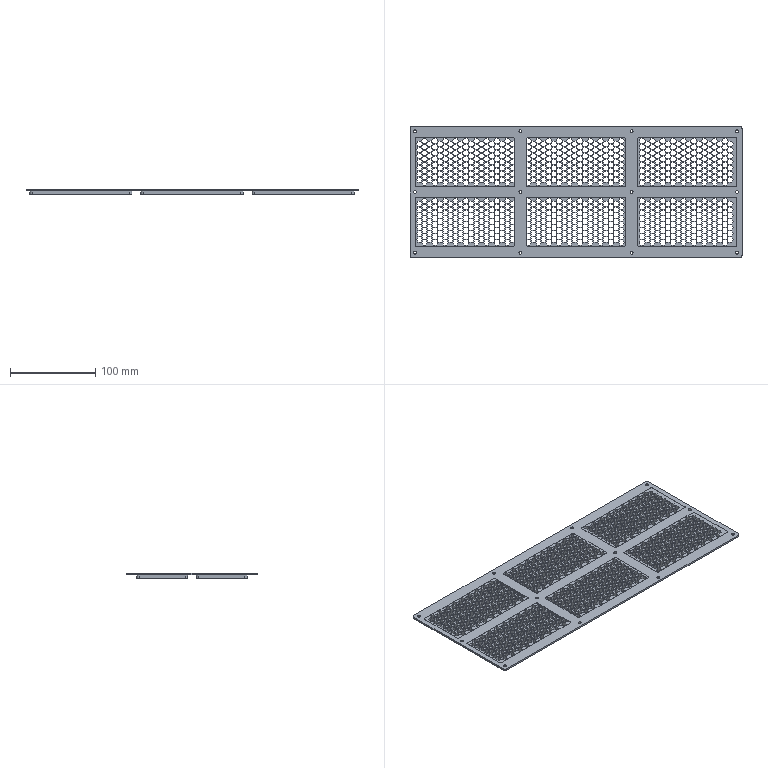NC program | NX | posted with a generic post
Lines 6817 to 7861 of 7861:
(DRILLING_1 , TOOL : D4)
N8550 T06 M6
N8552 G54
N8554 G17 G0 G90 X-183.338 Y14.437 S3000 M3
N8556 G43 Z10. H6
N8558 G94 G83 G98 Z-12.1 F200. Q5. R2.9
N8560 Y21.437
N8562 Y28.437
N8564 Y35.437
N8566 X-177.276 Y38.937
N8568 X-183.338 Y42.437
N8570 Y49.437
N8572 Y56.437
N8574 X-177.276 Y59.937
N8576 X-171.218 Y56.437
N8578 X-177.276 Y52.937
N8580 X-171.218 Y49.437
N8582 X-177.276 Y45.937
N8584 X-171.218 Y42.437
N8586 Y35.437
N8588 X-177.276 Y31.937
N8590 X-171.218 Y28.437
N8592 X-177.276 Y24.937
N8594 X-171.218 Y21.437
N8596 X-177.276 Y17.937
N8598 Y10.937
N8600 X-171.218 Y14.437
N8602 X-165.156 Y10.937
N8604 X-159.098 Y14.437
N8606 X-165.156 Y17.937
N8608 X-159.098 Y21.437
N8610 X-165.156 Y24.937
N8612 X-159.098 Y28.437
N8614 X-165.156 Y31.937
N8616 X-159.098 Y35.437
N8618 X-165.156 Y38.937
N8620 X-159.098 Y42.437
N8622 X-165.156 Y45.937
N8624 X-159.098 Y49.437
N8626 X-165.156 Y52.937
N8628 Y59.937
N8630 X-159.098 Y56.437
N8632 X-153.036 Y59.937
N8634 Y52.937
N8636 Y45.937
N8638 X-146.978 Y49.437
N8640 Y56.437
N8642 X-140.916 Y59.937
N8644 Y52.937
N8646 X-134.858 Y56.437
N8648 X-128.796 Y59.937
N8650 Y52.937
N8652 X-134.858 Y49.437
N8654 X-140.916 Y45.937
N8656 X-146.978 Y42.437
N8658 X-153.036 Y38.937
N8660 X-146.978 Y35.437
N8662 X-153.036 Y31.937
N8664 X-146.978 Y28.437
N8666 X-153.036 Y24.937
N8668 X-146.978 Y21.437
N8670 X-153.036 Y17.937
N8672 Y10.937
N8674 X-146.978 Y14.437
N8676 X-140.916 Y10.937
N8678 Y17.937
N8680 X-134.858 Y14.437
N8682 X-128.796 Y10.937
N8684 X-122.738 Y14.437
N8686 X-128.796 Y17.937
N8688 X-134.858 Y21.437
N8690 X-140.916 Y24.937
N8692 X-134.858 Y28.437
N8694 X-140.916 Y31.937
N8696 X-134.858 Y35.437
N8698 X-140.916 Y38.937
N8700 X-134.858 Y42.437
N8702 X-128.796 Y45.937
N8704 X-122.738 Y42.437
N8706 X-128.796 Y38.937
N8708 X-122.738 Y35.437
N8710 X-128.796 Y31.937
N8712 X-122.738 Y28.437
N8714 X-128.796 Y24.937
N8716 X-122.738 Y21.437
N8718 X-116.676 Y24.937
N8720 Y17.937
N8722 Y10.937
N8724 X-110.618 Y14.437
N8726 X-104.556 Y10.937
N8728 X-98.498 Y14.437
N8730 X-104.556 Y17.937
N8732 X-110.618 Y21.437
N8734 X-104.556 Y24.937
N8736 X-98.498 Y21.437
N8738 Y28.437
N8740 X-92.436 Y31.937
N8742 X-86.378 Y28.437
N8744 X-92.436 Y24.937
N8746 X-86.378 Y21.437
N8748 X-92.436 Y17.937
N8750 Y10.937
N8752 X-86.378 Y14.437
N8754 X-80.316 Y10.937
N8756 Y17.937
N8758 Y24.937
N8760 Y31.937
N8762 Y38.937
N8764 X-86.378 Y35.437
N8766 X-92.436 Y38.937
N8768 X-86.378 Y42.437
N8770 X-80.316 Y45.937
N8772 X-86.378 Y49.437
N8774 X-92.436 Y45.937
N8776 X-98.498 Y49.437
N8778 X-104.556 Y52.937
N8780 Y45.937
N8782 X-98.498 Y42.437
N8784 X-104.556 Y38.937
N8786 X-98.498 Y35.437
N8788 X-104.556 Y31.937
N8790 X-110.618 Y28.437
N8792 X-116.676 Y31.937
N8794 X-110.618 Y35.437
N8796 X-116.676 Y38.937
N8798 X-110.618 Y42.437
N8800 X-116.676 Y45.937
N8802 X-110.618 Y49.437
N8804 X-116.676 Y52.937
N8806 X-122.738 Y49.437
N8808 Y56.437
N8810 X-116.676 Y59.937
N8812 X-110.618 Y56.437
N8814 X-104.556 Y59.937
N8816 X-98.498 Y56.437
N8818 X-92.436 Y59.937
N8820 Y52.937
N8822 X-86.378 Y56.437
N8824 X-80.316 Y52.937
N8826 Y59.937
N8828 X-74.218 Y56.437
N8830 Y49.437
N8832 Y42.437
N8834 Y35.437
N8836 Y28.437
N8838 Y21.437
N8840 Y14.437
N8842 G80
N8844 G0 X-74.218 Y14.437 Z10.
(DRILLING_2 , TOOL : D4)
N8846 Z19.9
N8848 X-171.218 Y-48.563
N8850 G83 Z-12.1 F200. Q5. R2.9
N8852 X-177.276 Y-45.063
N8854 X-171.218 Y-41.563
N8856 X-177.276 Y-38.063
N8858 X-171.218 Y-34.563
N8860 X-177.276 Y-31.063
N8862 X-171.218 Y-27.563
N8864 X-177.276 Y-24.063
N8866 X-171.218 Y-20.563
N8868 X-177.276 Y-17.063
N8870 X-171.218 Y-13.563
N8872 X-177.276 Y-10.063
N8874 X-183.338 Y-13.563
N8876 Y-20.563
N8878 Y-27.563
N8880 Y-34.563
N8882 Y-41.563
N8884 Y-48.563
N8886 Y-55.563
N8888 X-177.276 Y-59.063
N8890 X-171.218 Y-55.563
N8892 X-165.156 Y-59.063
N8894 X-159.098 Y-55.563
N8896 X-165.156 Y-52.063
N8898 X-159.098 Y-48.563
N8900 X-165.156 Y-45.063
N8902 X-159.098 Y-41.563
N8904 X-165.156 Y-38.063
N8906 X-159.098 Y-34.563
N8908 X-165.156 Y-31.063
N8910 X-159.098 Y-27.563
N8912 X-165.156 Y-24.063
N8914 X-159.098 Y-20.563
N8916 X-165.156 Y-17.063
N8918 Y-10.063
N8920 X-159.098 Y-13.563
N8922 X-153.036 Y-10.063
N8924 X-146.978 Y-13.563
N8926 X-153.036 Y-17.063
N8928 X-146.978 Y-20.563
N8930 X-153.036 Y-24.063
N8932 X-146.978 Y-27.563
N8934 X-153.036 Y-31.063
N8936 X-146.978 Y-34.563
N8938 X-153.036 Y-38.063
N8940 X-146.978 Y-41.563
N8942 X-153.036 Y-45.063
N8944 X-146.978 Y-48.563
N8946 X-153.036 Y-52.063
N8948 Y-59.063
N8950 X-146.978 Y-55.563
N8952 X-140.916 Y-59.063
N8954 X-134.858 Y-55.563
N8956 X-140.916 Y-52.063
N8958 X-134.858 Y-48.563
N8960 X-140.916 Y-45.063
N8962 X-134.858 Y-41.563
N8964 X-140.916 Y-38.063
N8966 X-134.858 Y-34.563
N8968 X-140.916 Y-31.063
N8970 X-134.858 Y-27.563
N8972 X-140.916 Y-24.063
N8974 X-134.858 Y-20.563
N8976 X-140.916 Y-17.063
N8978 Y-10.063
N8980 X-134.858 Y-13.563
N8982 X-128.796 Y-10.063
N8984 X-122.738 Y-13.563
N8986 X-128.796 Y-17.063
N8988 X-122.738 Y-20.563
N8990 X-128.796 Y-24.063
N8992 X-122.738 Y-27.563
N8994 X-128.796 Y-31.063
N8996 X-122.738 Y-34.563
N8998 X-128.796 Y-38.063
N9000 X-122.738 Y-41.563
N9002 X-128.796 Y-45.063
N9004 X-122.738 Y-48.563
N9006 X-128.796 Y-52.063
N9008 Y-59.063
N9010 X-122.738 Y-55.563
N9012 X-116.676 Y-59.063
N9014 X-110.618 Y-55.563
N9016 X-116.676 Y-52.063
N9018 X-110.618 Y-48.563
N9020 X-116.676 Y-45.063
N9022 X-110.618 Y-41.563
N9024 X-116.676 Y-38.063
N9026 X-110.618 Y-34.563
N9028 X-116.676 Y-31.063
N9030 X-110.618 Y-27.563
N9032 X-116.676 Y-24.063
N9034 X-110.618 Y-20.563
N9036 X-116.676 Y-17.063
N9038 Y-10.063
N9040 X-110.618 Y-13.563
N9042 X-104.556 Y-10.063
N9044 X-98.498 Y-13.563
N9046 X-104.556 Y-17.063
N9048 X-98.498 Y-20.563
N9050 X-104.556 Y-24.063
N9052 X-98.498 Y-27.563
N9054 X-104.556 Y-31.063
N9056 X-98.498 Y-34.563
N9058 X-104.556 Y-38.063
N9060 X-98.498 Y-41.563
N9062 X-104.556 Y-45.063
N9064 X-98.498 Y-48.563
N9066 X-104.556 Y-52.063
N9068 Y-59.063
N9070 X-98.498 Y-55.563
N9072 X-92.436 Y-59.063
N9074 X-86.378 Y-55.563
N9076 X-92.436 Y-52.063
N9078 X-86.378 Y-48.563
N9080 X-92.436 Y-45.063
N9082 X-86.378 Y-41.563
N9084 X-92.436 Y-38.063
N9086 X-86.378 Y-34.563
N9088 X-92.436 Y-31.063
N9090 X-86.378 Y-27.563
N9092 X-80.316 Y-31.063
N9094 Y-38.063
N9096 Y-45.063
N9098 Y-52.063
N9100 Y-59.063
N9102 X-74.218 Y-55.563
N9104 Y-48.563
N9106 Y-41.563
N9108 Y-34.563
N9110 Y-27.563
N9112 Y-20.563
N9114 Y-13.563
N9116 X-80.316 Y-10.063
N9118 Y-17.063
N9120 Y-24.063
N9122 X-86.378 Y-20.563
N9124 X-92.436 Y-24.063
N9126 Y-17.063
N9128 X-86.378 Y-13.563
N9130 X-92.436 Y-10.063
N9132 X-177.276 Y-52.063
N9134 G80
N9136 G0 X-177.276 Y-52.063 Z19.9
(DRILLING_3 , TOOL : D4)
N9138 X-43.908 Y-45.063
N9140 G43 Z2.9 H6
N9142 G83 Z-12.1 F200. Q5. R2.9
N9144 X-37.85 Y-48.563
N9146 X-43.908 Y-52.063
N9148 X-37.85 Y-55.563
N9150 X-43.908 Y-59.063
N9152 X-49.97 Y-55.563
N9154 X-56.032 Y-59.063
N9156 Y-52.063
N9158 X-49.97 Y-48.563
N9160 X-56.032 Y-45.063
N9162 X-49.97 Y-41.563
N9164 X-56.032 Y-38.063
N9166 Y-31.063
N9168 X-49.97 Y-34.563
N9170 Y-27.563
N9172 Y-20.563
N9174 X-56.032 Y-24.063
N9176 Y-17.063
N9178 Y-10.063
N9180 X-49.97 Y-13.563
N9182 X-43.908 Y-10.063
N9184 X-37.85 Y-13.563
N9186 X-43.908 Y-17.063
N9188 X-37.85 Y-20.563
N9190 X-43.908 Y-24.063
N9192 X-37.85 Y-27.563
N9194 Y-34.563
N9196 X-43.908 Y-31.063
N9198 Y-38.063
N9200 X-37.85 Y-41.563
N9202 X-31.788 Y-38.063
N9204 Y-45.063
N9206 X-25.73 Y-41.563
N9208 Y-34.563
N9210 X-31.788 Y-31.063
N9212 X-25.73 Y-27.563
N9214 X-31.788 Y-24.063
N9216 X-25.73 Y-20.563
N9218 X-31.788 Y-17.063
N9220 Y-10.063
N9222 X-25.73 Y-13.563
N9224 X-19.668 Y-10.063
N9226 X-13.61 Y-13.563
N9228 X-19.668 Y-17.063
N9230 X-13.61 Y-20.563
N9232 X-19.668 Y-24.063
N9234 X-13.61 Y-27.563
N9236 X-19.668 Y-31.063
N9238 X-13.61 Y-34.563
N9240 X-19.668 Y-38.063
N9242 X-13.61 Y-41.563
N9244 X-19.668 Y-45.063
N9246 X-13.61 Y-48.563
N9248 X-19.668 Y-52.063
N9250 X-25.73 Y-48.563
N9252 X-31.788 Y-52.063
N9254 Y-59.063
N9256 X-25.73 Y-55.563
N9258 X-19.668 Y-59.063
N9260 X-13.61 Y-55.563
N9262 X-7.548 Y-52.063
N9264 Y-59.063
N9266 X-1.49 Y-55.563
N9268 X4.572 Y-59.063
N9270 X10.63 Y-55.563
N9272 X4.572 Y-52.063
N9274 X10.63 Y-48.563
N9276 X4.572 Y-45.063
N9278 X-1.49 Y-48.563
N9280 X-7.548 Y-45.063
N9282 X-1.49 Y-41.563
N9284 X-7.548 Y-38.063
N9286 X-1.49 Y-34.563
N9288 X-7.548 Y-31.063
N9290 X-1.49 Y-27.563
N9292 X4.572 Y-31.063
N9294 X10.63 Y-34.563
N9296 X4.572 Y-38.063
N9298 X10.63 Y-41.563
N9300 X16.692 Y-45.063
N9302 X22.75 Y-48.563
N9304 X16.692 Y-52.063
N9306 Y-59.063
N9308 X22.75 Y-55.563
N9310 X28.812 Y-59.063
N9312 X34.87 Y-55.563
N9314 X28.812 Y-52.063
N9316 X34.87 Y-48.563
N9318 X28.812 Y-45.063
N9320 X34.87 Y-41.563
N9322 X28.812 Y-38.063
N9324 X34.87 Y-34.563
N9326 X28.812 Y-31.063
N9328 X22.75 Y-34.563
N9330 Y-41.563
N9332 X16.692 Y-38.063
N9334 Y-31.063
N9336 X10.63 Y-27.563
N9338 X4.572 Y-24.063
N9340 X10.63 Y-20.563
N9342 X4.572 Y-17.063
N9344 X-1.49 Y-20.563
N9346 X-7.548 Y-24.063
N9348 Y-17.063
N9350 Y-10.063
N9352 X-1.49 Y-13.563
N9354 X4.572 Y-10.063
N9356 X10.63 Y-13.563
N9358 X16.692 Y-10.063
N9360 Y-17.063
N9362 X22.75 Y-13.563
N9364 X28.812 Y-10.063
N9366 X34.87 Y-13.563
N9368 X28.812 Y-17.063
N9370 X22.75 Y-20.563
N9372 X16.692 Y-24.063
N9374 X22.75 Y-27.563
N9376 X28.812 Y-24.063
N9378 X34.87 Y-20.563
N9380 Y-27.563
N9382 X40.932 Y-31.063
N9384 Y-38.063
N9386 X46.99 Y-41.563
N9388 X40.932 Y-45.063
N9390 Y-52.063
N9392 Y-59.063
N9394 X46.99 Y-55.563
N9396 X53.052 Y-59.063
N9398 Y-52.063
N9400 X46.99 Y-48.563
N9402 X53.052 Y-45.063
N9404 Y-38.063
N9406 X46.99 Y-34.563
N9408 X53.052 Y-31.063
N9410 Y-24.063
N9412 X46.99 Y-27.563
N9414 X40.932 Y-24.063
N9416 Y-17.063
N9418 X46.99 Y-20.563
N9420 X53.052 Y-17.063
N9422 Y-10.063
N9424 X46.99 Y-13.563
N9426 X40.932 Y-10.063
N9428 Y10.937
N9430 X34.87 Y14.437
N9432 X28.812 Y17.937
N9434 Y10.937
N9436 X22.75 Y14.437
N9438 X16.692 Y10.937
N9440 X10.63 Y14.437
N9442 X4.572 Y10.937
N9444 Y17.937
N9446 X10.63 Y21.437
N9448 X4.572 Y24.937
N9450 X10.63 Y28.437
N9452 X16.692 Y24.937
N9454 Y17.937
N9456 X22.75 Y21.437
N9458 Y28.437
N9460 Y35.437
N9462 X16.692 Y31.937
N9464 X10.63 Y35.437
N9466 X4.572 Y31.937
N9468 X-1.49 Y35.437
N9470 X4.572 Y38.937
N9472 X10.63 Y42.437
N9474 X16.692 Y45.937
N9476 Y38.937
N9478 X22.75 Y42.437
N9480 X28.812 Y38.937
N9482 Y45.937
N9484 X22.75 Y49.437
N9486 X28.812 Y52.937
N9488 X34.87 Y49.437
N9490 Y42.437
N9492 X40.932 Y38.937
N9494 Y31.937
N9496 X34.87 Y35.437
N9498 X28.812 Y31.937
N9500 X34.87 Y28.437
N9502 X28.812 Y24.937
N9504 X34.87 Y21.437
N9506 X40.932 Y24.937
N9508 Y17.937
N9510 X46.99 Y14.437
N9512 X53.052 Y10.937
N9514 Y17.937
N9516 X46.99 Y21.437
N9518 Y28.437
N9520 X53.052 Y24.937
N9522 Y31.937
N9524 X46.99 Y35.437
N9526 X53.052 Y38.937
N9528 X46.99 Y42.437
N9530 X53.052 Y45.937
N9532 Y52.937
N9534 Y59.937
N9536 X46.99 Y56.437
N9538 Y49.437
N9540 X40.932 Y45.937
N9542 Y52.937
N9544 Y59.937
N9546 X34.87 Y56.437
N9548 X28.812 Y59.937
N9550 X22.75 Y56.437
N9552 X16.692 Y59.937
N9554 Y52.937
N9556 X10.63 Y56.437
N9558 Y49.437
N9560 X4.572 Y45.937
N9562 Y52.937
N9564 Y59.937
N9566 X-1.49 Y56.437
N9568 X-7.548 Y59.937
N9570 X-13.61 Y56.437
N9572 X-7.548 Y52.937
N9574 X-1.49 Y49.437
N9576 X-7.548 Y45.937
N9578 X-1.49 Y42.437
N9580 X-7.548 Y38.937
N9582 X-13.61 Y35.437
N9584 X-19.668 Y31.937
N9586 Y38.937
N9588 X-13.61 Y42.437
N9590 X-19.668 Y45.937
N9592 X-13.61 Y49.437
N9594 X-19.668 Y52.937
N9596 Y59.937
N9598 X-25.73 Y56.437
N9600 Y49.437
N9602 X-31.788 Y52.937
N9604 Y59.937
N9606 X-37.85 Y56.437
N9608 X-43.908 Y59.937
N9610 Y52.937
N9612 Y45.937
N9614 X-49.97 Y49.437
N9616 Y56.437
N9618 X-56.032 Y59.937
N9620 Y52.937
N9622 Y45.937
N9624 Y38.937
N9626 X-49.97 Y42.437
N9628 Y35.437
N9630 X-56.032 Y31.937
N9632 Y24.937
N9634 X-49.97 Y28.437
N9636 X-43.908 Y31.937
N9638 X-37.85 Y35.437
N9640 X-43.908 Y38.937
N9642 X-37.85 Y42.437
N9644 Y49.437
N9646 X-31.788 Y45.937
N9648 X-25.73 Y42.437
N9650 X-31.788 Y38.937
N9652 X-25.73 Y35.437
N9654 X-31.788 Y31.937
N9656 X-25.73 Y28.437
N9658 X-31.788 Y24.937
N9660 X-25.73 Y21.437
N9662 X-31.788 Y17.937
N9664 X-37.85 Y21.437
N9666 Y28.437
N9668 X-43.908 Y24.937
N9670 X-49.97 Y21.437
N9672 X-56.032 Y17.937
N9674 Y10.937
N9676 X-49.97 Y14.437
N9678 X-43.908 Y17.937
N9680 Y10.937
N9682 X-37.85 Y14.437
N9684 X-31.788 Y10.937
N9686 X-25.73 Y14.437
N9688 X-19.668 Y10.937
N9690 X-13.61 Y14.437
N9692 X-19.668 Y17.937
N9694 X-13.61 Y21.437
N9696 X-19.668 Y24.937
N9698 X-13.61 Y28.437
N9700 X-7.548 Y31.937
N9702 X-1.49 Y28.437
N9704 X-7.548 Y24.937
N9706 X-1.49 Y21.437
N9708 X-7.548 Y17.937
N9710 X-1.49 Y14.437
N9712 X-7.548 Y10.937
N9714 G80
(DRILLING_4 , TOOL : D4)
N9716 G83 G99 X107.673 Y42.437 Z-12.1 F200. Q5. R2.9
N9718 X113.731 Y38.937
N9720 X107.673 Y35.437
N9722 X113.731 Y31.937
N9724 Y24.937
N9726 X107.673 Y28.437
N9728 X101.611 Y24.937
N9730 X107.673 Y21.437
N9732 X113.731 Y17.937
N9734 Y10.937
N9736 X107.673 Y14.437
N9738 X101.611 Y17.937
N9740 Y10.937
N9742 X95.553 Y14.437
N9744 X89.491 Y17.937
N9746 Y10.937
N9748 X83.433 Y14.437
N9750 X77.371 Y10.937
N9752 Y17.937
N9754 X83.433 Y21.437
N9756 X77.371 Y24.937
N9758 Y31.937
N9760 Y38.937
N9762 Y45.937
N9764 Y52.937
N9766 Y59.937
N9768 X83.433 Y56.437
N9770 X89.491 Y59.937
N9772 Y52.937
N9774 X83.433 Y49.437
N9776 X89.491 Y45.937
N9778 X83.433 Y42.437
N9780 X89.491 Y38.937
N9782 X83.433 Y35.437
N9784 X89.491 Y31.937
N9786 X83.433 Y28.437
N9788 X89.491 Y24.937
N9790 X95.553 Y21.437
N9792 Y28.437
N9794 X101.611 Y31.937
N9796 X95.553 Y35.437
N9798 X101.611 Y38.937
N9800 X95.553 Y42.437
N9802 X101.611 Y45.937
N9804 X95.553 Y49.437
N9806 X101.611 Y52.937
N9808 X95.553 Y56.437
N9810 X101.611 Y59.937
N9812 X107.673 Y56.437
N9814 X113.731 Y59.937
N9816 Y52.937
N9818 X107.673 Y49.437
N9820 X113.731 Y45.937
N9822 X119.793 Y49.437
N9824 Y56.437
N9826 X125.851 Y59.937
N9828 Y52.937
N9830 X131.913 Y49.437
N9832 X137.971 Y52.937
N9834 X131.913 Y56.437
N9836 X137.971 Y59.937
N9838 X144.033 Y56.437
N9840 X150.091 Y59.937
N9842 Y52.937
N9844 X144.033 Y49.437
N9846 X137.971 Y45.937
N9848 X144.033 Y42.437
N9850 X150.091 Y38.937
N9852 Y31.937
N9854 Y24.937
N9856 X144.033 Y28.437
N9858 Y35.437
N9860 X137.971 Y38.937
N9862 Y31.937
N9864 Y24.937
N9866 X144.033 Y21.437
N9868 X150.091 Y17.937
N9870 X156.153 Y21.437
N9872 Y28.437
N9874 X162.211 Y31.937
N9876 X156.153 Y35.437
N9878 X162.211 Y38.937
N9880 X156.153 Y42.437
N9882 X150.091 Y45.937
N9884 X156.153 Y49.437
N9886 Y56.437
N9888 X162.211 Y59.937
N9890 X168.273 Y56.437
N9892 Y49.437
N9894 X162.211 Y52.937
N9896 Y45.937
N9898 X168.273 Y42.437
N9900 Y35.437
N9902 X174.331 Y38.937
N9904 Y45.937
N9906 Y52.937
N9908 Y59.937
N9910 X180.393 Y56.437
N9912 Y49.437
N9914 Y42.437
N9916 Y35.437
N9918 X174.331 Y31.937
N9920 Y24.937
N9922 X180.393 Y28.437
N9924 Y21.437
N9926 Y14.437
N9928 X174.331 Y17.937
N9930 Y10.937
N9932 X168.273 Y14.437
N9934 Y21.437
N9936 Y28.437
N9938 X162.211 Y24.937
N9940 Y17.937
N9942 Y10.937
N9944 X156.153 Y14.437
N9946 X150.091 Y10.937
N9948 X144.033 Y14.437
N9950 X137.971 Y10.937
N9952 X131.913 Y14.437
N9954 X137.971 Y17.937
N9956 X131.913 Y21.437
N9958 Y28.437
N9960 Y35.437
N9962 Y42.437
N9964 X125.851 Y45.937
N9966 X119.793 Y42.437
N9968 X125.851 Y38.937
N9970 X119.793 Y35.437
N9972 X125.851 Y31.937
N9974 X119.793 Y28.437
N9976 X125.851 Y24.937
N9978 X119.793 Y21.437
N9980 X125.851 Y17.937
N9982 X119.793 Y14.437
N9984 X125.851 Y10.937
N9986 X137.971 Y-10.063
N9988 X131.913 Y-13.563
N9990 X125.851 Y-10.063
N9992 X119.793 Y-13.563
N9994 X125.851 Y-17.063
N9996 X119.793 Y-20.563
N9998 X125.851 Y-24.063
N10000 X119.793 Y-27.563
N10002 X125.851 Y-31.063
N10004 X119.793 Y-34.563
N10006 X113.731 Y-38.063
N10008 X107.673 Y-34.563
N10010 X113.731 Y-31.063
N10012 X107.673 Y-27.563
N10014 X113.731 Y-24.063
N10016 X107.673 Y-20.563
N10018 X113.731 Y-17.063
N10020 Y-10.063
N10022 X107.673 Y-13.563
N10024 X101.611 Y-10.063
N10026 X95.553 Y-13.563
N10028 X101.611 Y-17.063
N10030 X95.553 Y-20.563
N10032 X101.611 Y-24.063
N10034 X95.553 Y-27.563
N10036 X89.491 Y-24.063
N10038 X83.433 Y-20.563
N10040 X89.491 Y-17.063
N10042 Y-10.063
N10044 X83.433 Y-13.563
N10046 X77.371 Y-10.063
N10048 Y-17.063
N10050 Y-24.063
N10052 Y-31.063
N10054 X83.433 Y-27.563
N10056 X89.491 Y-31.063
N10058 X83.433 Y-34.563
N10060 X77.371 Y-38.063
N10062 Y-45.063
N10064 Y-52.063
N10066 Y-59.063
N10068 X83.433 Y-55.563
N10070 X89.491 Y-59.063
N10072 Y-52.063
N10074 X83.433 Y-48.563
N10076 X89.491 Y-45.063
N10078 X83.433 Y-41.563
N10080 X89.491 Y-38.063
N10082 X95.553 Y-34.563
N10084 X101.611 Y-31.063
N10086 Y-38.063
N10088 X95.553 Y-41.563
N10090 X101.611 Y-45.063
N10092 X95.553 Y-48.563
N10094 X101.611 Y-52.063
N10096 X95.553 Y-55.563
N10098 X101.611 Y-59.063
N10100 X107.673 Y-55.563
N10102 X113.731 Y-59.063
N10104 Y-52.063
N10106 X107.673 Y-48.563
N10108 Y-41.563
N10110 X113.731 Y-45.063
N10112 X119.793 Y-48.563
N10114 X125.851 Y-45.063
N10116 X119.793 Y-41.563
N10118 X125.851 Y-38.063
N10120 X131.913 Y-41.563
N10122 X137.971 Y-38.063
N10124 X131.913 Y-34.563
N10126 X137.971 Y-31.063
N10128 X131.913 Y-27.563
N10130 Y-20.563
N10132 X137.971 Y-24.063
N10134 X144.033 Y-27.563
N10136 X150.091 Y-31.063
N10138 X144.033 Y-34.563
N10140 X150.091 Y-38.063
N10142 X156.153 Y-34.563
N10144 X162.211 Y-38.063
N10146 X168.273 Y-34.563
N10148 X162.211 Y-31.063
N10150 X156.153 Y-27.563
N10152 X150.091 Y-24.063
N10154 X144.033 Y-20.563
N10156 X137.971 Y-17.063
N10158 X144.033 Y-13.563
N10160 X150.091 Y-10.063
N10162 Y-17.063
N10164 X156.153 Y-20.563
N10166 X162.211 Y-24.063
N10168 Y-17.063
N10170 X156.153 Y-13.563
N10172 X162.211 Y-10.063
N10174 X168.273 Y-13.563
N10176 X174.331 Y-10.063
N10178 X180.393 Y-13.563
N10180 Y-20.563
N10182 X174.331 Y-17.063
N10184 Y-24.063
N10186 X168.273 Y-20.563
N10188 Y-27.563
N10190 X174.331 Y-31.063
N10192 X180.393 Y-27.563
N10194 Y-34.563
N10196 X174.331 Y-38.063
N10198 X180.393 Y-41.563
N10200 Y-48.563
N10202 Y-55.563
N10204 X174.331 Y-59.063
N10206 Y-52.063
N10208 X168.273 Y-48.563
N10210 X174.331 Y-45.063
N10212 X168.273 Y-41.563
N10214 X162.211 Y-45.063
N10216 X156.153 Y-41.563
N10218 Y-48.563
N10220 X162.211 Y-52.063
N10222 X168.273 Y-55.563
N10224 X162.211 Y-59.063
N10226 X156.153 Y-55.563
N10228 X150.091 Y-59.063
N10230 X144.033 Y-55.563
N10232 X150.091 Y-52.063
N10234 X144.033 Y-48.563
N10236 X150.091 Y-45.063
N10238 X144.033 Y-41.563
N10240 X137.971 Y-45.063
N10242 Y-52.063
N10244 X131.913 Y-48.563
N10246 X125.851 Y-52.063
N10248 X119.793 Y-55.563
N10250 X125.851 Y-59.063
N10252 X131.913 Y-55.563
N10254 X137.971 Y-59.063
N10256 G80
N10258 M5
(PLANAR_MILL_1_COPY_1 , TOOL : D4_ROUGH)
N10260 T07 M6
N10262 G54
N10264 G17 G43 G0 G90 X-71.888 Y-79.75 S5500 H7 M3
N10266 Z43.
N10268 Z-6.
N10270 G94 G1 X-192.088 Z-6.063 F2000.
N10272 X-193.619 Y-79.378 Z-6.064
N10274 X-194.992 Y-78.606 Z-6.065
N10276 X-196.106 Y-77.492
N10278 X-196.878 Y-76.119 Z-6.066
N10280 X-197.25 Y-74.588 Z-6.067
N10282 Y74.588 Z-6.145
N10284 X-196.878 Y76.119 Z-6.146
N10286 X-196.106 Y77.492 Z-6.147
N10288 X-194.992 Y78.606 Z-6.148
N10290 X-193.619 Y79.378
N10292 X-192.088 Y79.75 Z-6.149
N10294 X192.088 Z-6.35
N10296 X193.619 Y79.378 Z-6.351
N10298 X194.992 Y78.606 Z-6.352
N10300 X196.106 Y77.492 Z-6.353
N10302 X196.878 Y76.119 Z-6.354
N10304 X197.25 Y74.588 Z-6.355
N10306 Y-74.588 Z-6.433
N10308 X196.878 Y-76.119 Z-6.434
N10310 X196.106 Y-77.492
N10312 X194.992 Y-78.606 Z-6.435
N10314 X193.619 Y-79.378 Z-6.436
N10316 X192.088 Y-79.75 Z-6.437
N10318 X-192.088 Z-6.638
N10320 X-193.619 Y-79.378 Z-6.639
N10322 X-194.992 Y-78.606 Z-6.64
N10324 X-196.106 Y-77.492
N10326 X-196.878 Y-76.119 Z-6.641
N10328 X-197.25 Y-74.588 Z-6.642
N10330 Y74.588 Z-6.72
N10332 X-196.878 Y76.119 Z-6.721
N10334 X-196.106 Y77.492 Z-6.722
N10336 X-194.992 Y78.606 Z-6.723
N10338 X-193.619 Y79.378
N10340 X-192.088 Y79.75 Z-6.724
N10342 X192.088 Z-6.925
N10344 X193.619 Y79.378 Z-6.926
N10346 X194.992 Y78.606 Z-6.927
N10348 X196.106 Y77.492 Z-6.928
N10350 X196.878 Y76.119 Z-6.929
N10352 X197.25 Y74.588 Z-6.93
N10354 Y-74.588 Z-7.008
N10356 X196.878 Y-76.119 Z-7.009
N10358 X196.106 Y-77.492
N10360 X194.992 Y-78.606 Z-7.01
N10362 X193.619 Y-79.378 Z-7.011
N10364 X192.088 Y-79.75 Z-7.012
N10366 X-192.088 Z-7.213
N10368 X-193.619 Y-79.378 Z-7.214
N10370 X-194.992 Y-78.606 Z-7.215
N10372 X-196.106 Y-77.492
N10374 X-196.878 Y-76.119 Z-7.216
N10376 X-197.25 Y-74.588 Z-7.217
N10378 Y74.588 Z-7.295
N10380 X-196.878 Y76.119 Z-7.296
N10382 X-196.106 Y77.492 Z-7.297
N10384 X-194.992 Y78.606 Z-7.298
N10386 X-193.619 Y79.378 Z-7.299
N10388 X-192.088 Y79.75
N10390 X192.088 Z-7.5
N10392 X193.619 Y79.378 Z-7.501
N10394 X194.992 Y78.606 Z-7.502
N10396 X196.106 Y77.492 Z-7.503
N10398 X196.878 Y76.119 Z-7.504
N10400 X197.25 Y74.588 Z-7.505
N10402 Y-74.588 Z-7.583
N10404 X196.878 Y-76.119 Z-7.584
N10406 X196.106 Y-77.492
N10408 X194.992 Y-78.606 Z-7.585
N10410 X193.619 Y-79.378 Z-7.586
N10412 X192.088 Y-79.75 Z-7.587
N10414 X-192.088 Z-7.788
N10416 X-193.619 Y-79.378 Z-7.789
N10418 X-194.992 Y-78.606 Z-7.79
N10420 X-196.106 Y-77.492
N10422 X-196.878 Y-76.119 Z-7.791
N10424 X-197.25 Y-74.588 Z-7.792
N10426 Y74.588 Z-7.87
N10428 X-196.878 Y76.119 Z-7.871
N10430 X-196.106 Y77.492 Z-7.872
N10432 X-194.992 Y78.606 Z-7.873
N10434 X-193.619 Y79.378 Z-7.874
N10436 X-192.088 Y79.75
N10438 X192.088 Z-8.076
N10440 X193.619 Y79.378
N10442 X194.992 Y78.606 Z-8.077
N10444 X196.106 Y77.492 Z-8.078
N10446 X196.878 Y76.119 Z-8.079
N10448 X197.25 Y74.588 Z-8.08
N10450 Y-74.588 Z-8.158
N10452 X196.878 Y-76.119 Z-8.159
N10454 X196.106 Y-77.492
N10456 X194.992 Y-78.606 Z-8.16
N10458 X193.619 Y-79.378 Z-8.161
N10460 X192.088 Y-79.75 Z-8.162
N10462 X-192.088 Z-8.363
N10464 X-193.619 Y-79.378 Z-8.364
N10466 X-194.992 Y-78.606 Z-8.365
N10468 X-196.106 Y-77.492
N10470 X-196.878 Y-76.119 Z-8.366
N10472 X-197.25 Y-74.588 Z-8.367
N10474 Y74.588 Z-8.445
N10476 X-196.878 Y76.119 Z-8.446
N10478 X-196.106 Y77.492 Z-8.447
N10480 X-194.992 Y78.606 Z-8.448
N10482 X-193.619 Y79.378 Z-8.449
N10484 X-192.088 Y79.75
N10486 X192.088 Z-8.651
N10488 X193.619 Y79.378
N10490 X194.992 Y78.606 Z-8.652
N10492 X196.106 Y77.492 Z-8.653
N10494 X196.878 Y76.119 Z-8.654
N10496 X197.25 Y74.588 Z-8.655
N10498 Y-74.588 Z-8.733
N10500 X196.878 Y-76.119 Z-8.734
N10502 X196.106 Y-77.492
N10504 X194.992 Y-78.606 Z-8.735
N10506 X193.619 Y-79.378 Z-8.736
N10508 X192.088 Y-79.75 Z-8.737
N10510 X-192.088 Z-8.938
N10512 X-193.619 Y-79.378 Z-8.939
N10514 X-194.992 Y-78.606 Z-8.94
N10516 X-196.106 Y-77.492 Z-8.941
N10518 X-196.878 Y-76.119
N10520 X-197.25 Y-74.588 Z-8.942
N10522 Y74.588 Z-9.02
N10524 X-196.878 Y76.119 Z-9.021
N10526 X-196.106 Y77.492 Z-9.022
N10528 X-194.992 Y78.606 Z-9.023
N10530 X-193.619 Y79.378 Z-9.024
N10532 X-192.088 Y79.75
N10534 X192.088 Z-9.226
N10536 X193.619 Y79.378
N10538 X194.992 Y78.606 Z-9.227
N10540 X196.106 Y77.492 Z-9.228
N10542 X196.878 Y76.119 Z-9.229
N10544 X197.25 Y74.588 Z-9.23
N10546 Y-74.588 Z-9.308
N10548 X196.878 Y-76.119 Z-9.309
N10550 X196.106 Y-77.492
N10552 X194.992 Y-78.606 Z-9.31
N10554 X193.619 Y-79.378 Z-9.311
N10556 X192.088 Y-79.75 Z-9.312
N10558 X-192.088 Z-9.513
N10560 X-193.619 Y-79.378 Z-9.514
N10562 X-194.992 Y-78.606 Z-9.515
N10564 X-196.106 Y-77.492 Z-9.516
N10566 X-196.878 Y-76.119
N10568 X-197.25 Y-74.588 Z-9.517
N10570 Y74.588 Z-9.595
N10572 X-196.878 Y76.119 Z-9.596
N10574 X-196.106 Y77.492 Z-9.597
N10576 X-194.992 Y78.606 Z-9.598
N10578 X-193.619 Y79.378 Z-9.599
N10580 X-192.088 Y79.75
N10582 X0. Z-9.7
N10584 X191.5
N10586 G2 X197.25 Y74. R5.75
N10588 G1 Y-74.
N10590 G2 X191.5 Y-79.75 R5.75
N10592 G1 X-191.5
N10594 G2 X-197.25 Y-74. R5.75
N10596 G1 Y74.
N10598 G2 X-191.5 Y79.75 R5.75
N10600 G1 X0.
N10602 Z-8.7
N10604 G0 Z43.
N10606 M5
N10608 M2